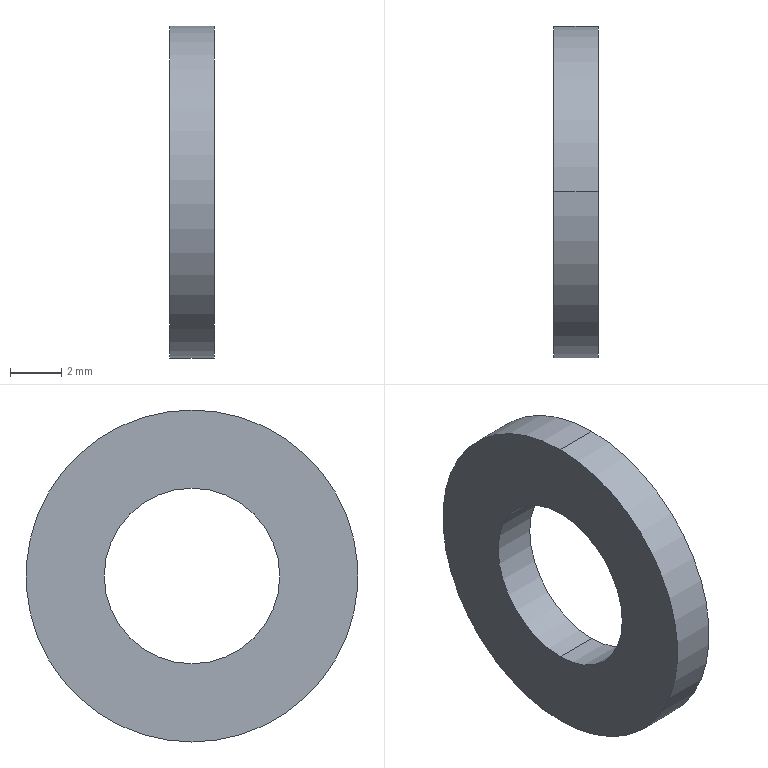Part | STEP file | flat washer narrow_am_B18.22M - Plain washer, 6 mm, narrow | 1 solid | 6 faces | box 1.75 x 13 x 13 mm | volume 167.412 mm3 | cylinder 4 | plane 2 | commonest cylinder face diameters 6.87 x2 13 x2
STEP:
#1=CARTESIAN_POINT('',(0.,0.,0.));
#2=DIRECTION('',(0.,0.,1.));
#3=DIRECTION('',(1.,0.,0.));
#4=AXIS2_PLACEMENT_3D('',#1,#2,#3);
#5=CARTESIAN_POINT('',(0.,0.,6.5));
#6=VERTEX_POINT('',#5);
#7=CARTESIAN_POINT('',(0.,0.,-6.5));
#8=VERTEX_POINT('',#7);
#9=CARTESIAN_POINT('',(0.,0.,0.));
#10=DIRECTION('',(-1.,0.,0.));
#11=DIRECTION('',(0.,0.,1.));
#12=AXIS2_PLACEMENT_3D('',#9,#10,#11);
#13=CIRCLE('',#12,6.5);
#14=CARTESIAN_POINT('',(-34.925,0.,0.));
#15=DIRECTION('',(-1.,0.,0.));
#16=DIRECTION('',(0.,0.,1.));
#17=AXIS2_PLACEMENT_3D('',#14,#15,#16);
#18=CYLINDRICAL_SURFACE('',#17,6.5);
#19=CARTESIAN_POINT('',(0.,-34.925));
#20=DIRECTION('',(1.,0.));
#21=VECTOR('',#20,1.);
#22=LINE('',#19,#21);
#23=(GEOMETRIC_REPRESENTATION_CONTEXT(2)PARAMETRIC_REPRESENTATION_CONTEXT()REPRESENTATION_CONTEXT('',''));
#24=DEFINITIONAL_REPRESENTATION('',(#22),#23);
#25=PCURVE('',#18,#24);
#26=CARTESIAN_POINT('',(0.,3.435,0.));
#27=DIRECTION('',(-1.,0.,0.));
#28=DIRECTION('',(0.,0.,1.));
#29=AXIS2_PLACEMENT_3D('',#26,#27,#28);
#30=PLANE('',#29);
#31=CARTESIAN_POINT('',(0.,-3.435));
#32=DIRECTION('',(1.,0.));
#33=AXIS2_PLACEMENT_2D('',#31,#32);
#34=CIRCLE('',#33,6.5);
#35=(GEOMETRIC_REPRESENTATION_CONTEXT(2)PARAMETRIC_REPRESENTATION_CONTEXT()REPRESENTATION_CONTEXT('',''));
#36=DEFINITIONAL_REPRESENTATION('',(#34),#35);
#37=PCURVE('',#30,#36);
#38=SURFACE_CURVE('',#13,(#25,#37),.PCURVE_S1.);
#39=EDGE_CURVE('',#6,#8,#38,.T.);
#40=ORIENTED_EDGE('',*,*,#39,.T.);
#41=CARTESIAN_POINT('',(-1.75,0.,-6.5));
#42=VERTEX_POINT('',#41);
#43=CARTESIAN_POINT('',(-34.925,0.,-6.5));
#44=DIRECTION('',(-1.,0.,0.));
#45=VECTOR('',#44,1.);
#46=LINE('',#43,#45);
#47=CARTESIAN_POINT('',(3.142,0.));
#48=DIRECTION('',(0.,1.));
#49=VECTOR('',#48,1.);
#50=LINE('',#47,#49);
#51=(GEOMETRIC_REPRESENTATION_CONTEXT(2)PARAMETRIC_REPRESENTATION_CONTEXT()REPRESENTATION_CONTEXT('',''));
#52=DEFINITIONAL_REPRESENTATION('',(#50),#51);
#53=PCURVE('',#18,#52);
#54=CARTESIAN_POINT('',(-34.925,0.,0.));
#55=DIRECTION('',(-1.,0.,0.));
#56=DIRECTION('',(0.,0.,1.));
#57=AXIS2_PLACEMENT_3D('',#54,#55,#56);
#58=CYLINDRICAL_SURFACE('',#57,6.5);
#59=CARTESIAN_POINT('',(3.142,0.));
#60=DIRECTION('',(0.,1.));
#61=VECTOR('',#60,1.);
#62=LINE('',#59,#61);
#63=(GEOMETRIC_REPRESENTATION_CONTEXT(2)PARAMETRIC_REPRESENTATION_CONTEXT()REPRESENTATION_CONTEXT('',''));
#64=DEFINITIONAL_REPRESENTATION('',(#62),#63);
#65=PCURVE('',#58,#64);
#66=SURFACE_CURVE('',#46,(#53,#65),.PCURVE_S1.);
#67=EDGE_CURVE('',#8,#42,#66,.T.);
#68=ORIENTED_EDGE('',*,*,#67,.T.);
#69=CARTESIAN_POINT('',(-1.75,0.,6.5));
#70=VERTEX_POINT('',#69);
#71=CARTESIAN_POINT('',(-1.75,0.,0.));
#72=DIRECTION('',(-1.,0.,0.));
#73=DIRECTION('',(0.,0.,1.));
#74=AXIS2_PLACEMENT_3D('',#71,#72,#73);
#75=CIRCLE('',#74,6.5);
#76=CARTESIAN_POINT('',(0.,-33.175));
#77=DIRECTION('',(1.,0.));
#78=VECTOR('',#77,1.);
#79=LINE('',#76,#78);
#80=(GEOMETRIC_REPRESENTATION_CONTEXT(2)PARAMETRIC_REPRESENTATION_CONTEXT()REPRESENTATION_CONTEXT('',''));
#81=DEFINITIONAL_REPRESENTATION('',(#79),#80);
#82=PCURVE('',#18,#81);
#83=CARTESIAN_POINT('',(-1.75,6.5,0.));
#84=DIRECTION('',(1.,0.,0.));
#85=DIRECTION('',(0.,0.,-1.));
#86=AXIS2_PLACEMENT_3D('',#83,#84,#85);
#87=PLANE('',#86);
#88=CARTESIAN_POINT('',(-6.5,-6.5));
#89=CARTESIAN_POINT('',(-6.5,4.758));
#90=CARTESIAN_POINT('',(3.25,-0.8708));
#91=CARTESIAN_POINT('',(13.,-6.5));
#92=CARTESIAN_POINT('',(3.25,-12.129));
#93=CARTESIAN_POINT('',(-6.5,-17.758));
#94=CARTESIAN_POINT('',(-6.5,-6.5));
#95=(BOUNDED_CURVE()B_SPLINE_CURVE(2,(#88,#89,#90,#91,#92,#93,#94),.UNSPECIFIED.,.T.,.F.)B_SPLINE_CURVE_WITH_KNOTS((1,2,2,2,2,1),(-2.094,0.,2.094,4.189,6.283,8.378),.UNSPECIFIED.)CURVE()GEOMETRIC_REPRESENTATION_ITEM()RATIONAL_B_SPLINE_CURVE((1.,0.5,1.,0.5,1.,0.5,1.))REPRESENTATION_ITEM(''));
#96=(GEOMETRIC_REPRESENTATION_CONTEXT(2)PARAMETRIC_REPRESENTATION_CONTEXT()REPRESENTATION_CONTEXT('',''));
#97=DEFINITIONAL_REPRESENTATION('',(#95),#96);
#98=PCURVE('',#87,#97);
#99=SURFACE_CURVE('',#75,(#82,#98),.PCURVE_S1.);
#100=EDGE_CURVE('',#70,#42,#99,.T.);
#101=ORIENTED_EDGE('',*,*,#100,.F.);
#102=CARTESIAN_POINT('',(-34.925,0.,6.5));
#103=DIRECTION('',(-1.,0.,0.));
#104=VECTOR('',#103,1.);
#105=LINE('',#102,#104);
#106=CARTESIAN_POINT('',(0.,0.));
#107=DIRECTION('',(0.,1.));
#108=VECTOR('',#107,1.);
#109=LINE('',#106,#108);
#110=(GEOMETRIC_REPRESENTATION_CONTEXT(2)PARAMETRIC_REPRESENTATION_CONTEXT()REPRESENTATION_CONTEXT('',''));
#111=DEFINITIONAL_REPRESENTATION('',(#109),#110);
#112=PCURVE('',#18,#111);
#113=CARTESIAN_POINT('',(6.283,0.));
#114=DIRECTION('',(0.,1.));
#115=VECTOR('',#114,1.);
#116=LINE('',#113,#115);
#117=(GEOMETRIC_REPRESENTATION_CONTEXT(2)PARAMETRIC_REPRESENTATION_CONTEXT()REPRESENTATION_CONTEXT('',''));
#118=DEFINITIONAL_REPRESENTATION('',(#116),#117);
#119=PCURVE('',#58,#118);
#120=SURFACE_CURVE('',#105,(#112,#119),.PCURVE_S1.);
#121=EDGE_CURVE('',#6,#70,#120,.T.);
#122=ORIENTED_EDGE('',*,*,#121,.F.);
#123=EDGE_LOOP('',(#40,#68,#101,#122));
#124=FACE_BOUND('',#123,.T.);
#125=ADVANCED_FACE('',(#124),#18,.T.);
#126=CARTESIAN_POINT('',(0.,0.,3.435));
#127=VERTEX_POINT('',#126);
#128=CARTESIAN_POINT('',(-1.75,0.,3.435));
#129=VERTEX_POINT('',#128);
#130=CARTESIAN_POINT('',(-34.925,0.,3.435));
#131=DIRECTION('',(-1.,0.,0.));
#132=VECTOR('',#131,1.);
#133=LINE('',#130,#132);
#134=CARTESIAN_POINT('',(-34.925,0.,0.));
#135=DIRECTION('',(-1.,0.,0.));
#136=DIRECTION('',(0.,0.,1.));
#137=AXIS2_PLACEMENT_3D('',#134,#135,#136);
#138=CYLINDRICAL_SURFACE('',#137,3.435);
#139=CARTESIAN_POINT('',(6.283,0.));
#140=DIRECTION('',(0.,1.));
#141=VECTOR('',#140,1.);
#142=LINE('',#139,#141);
#143=(GEOMETRIC_REPRESENTATION_CONTEXT(2)PARAMETRIC_REPRESENTATION_CONTEXT()REPRESENTATION_CONTEXT('',''));
#144=DEFINITIONAL_REPRESENTATION('',(#142),#143);
#145=PCURVE('',#138,#144);
#146=CARTESIAN_POINT('',(-34.925,0.,0.));
#147=DIRECTION('',(-1.,0.,0.));
#148=DIRECTION('',(0.,0.,1.));
#149=AXIS2_PLACEMENT_3D('',#146,#147,#148);
#150=CYLINDRICAL_SURFACE('',#149,3.435);
#151=CARTESIAN_POINT('',(0.,0.));
#152=DIRECTION('',(0.,1.));
#153=VECTOR('',#152,1.);
#154=LINE('',#151,#153);
#155=(GEOMETRIC_REPRESENTATION_CONTEXT(2)PARAMETRIC_REPRESENTATION_CONTEXT()REPRESENTATION_CONTEXT('',''));
#156=DEFINITIONAL_REPRESENTATION('',(#154),#155);
#157=PCURVE('',#150,#156);
#158=SURFACE_CURVE('',#133,(#145,#157),.PCURVE_S1.);
#159=EDGE_CURVE('',#127,#129,#158,.T.);
#160=ORIENTED_EDGE('',*,*,#159,.T.);
#161=CARTESIAN_POINT('',(-1.75,0.,-3.435));
#162=VERTEX_POINT('',#161);
#163=CARTESIAN_POINT('',(-1.75,0.,0.));
#164=DIRECTION('',(-1.,0.,0.));
#165=DIRECTION('',(0.,0.,1.));
#166=AXIS2_PLACEMENT_3D('',#163,#164,#165);
#167=CIRCLE('',#166,3.435);
#168=CARTESIAN_POINT('',(0.,-33.175));
#169=DIRECTION('',(1.,0.));
#170=VECTOR('',#169,1.);
#171=LINE('',#168,#170);
#172=(GEOMETRIC_REPRESENTATION_CONTEXT(2)PARAMETRIC_REPRESENTATION_CONTEXT()REPRESENTATION_CONTEXT('',''));
#173=DEFINITIONAL_REPRESENTATION('',(#171),#172);
#174=PCURVE('',#138,#173);
#175=CARTESIAN_POINT('',(-3.435,-6.5));
#176=CARTESIAN_POINT('',(-3.435,-0.5504));
#177=CARTESIAN_POINT('',(1.718,-3.525));
#178=CARTESIAN_POINT('',(6.87,-6.5));
#179=CARTESIAN_POINT('',(1.718,-9.475));
#180=CARTESIAN_POINT('',(-3.435,-12.45));
#181=CARTESIAN_POINT('',(-3.435,-6.5));
#182=(BOUNDED_CURVE()B_SPLINE_CURVE(2,(#175,#176,#177,#178,#179,#180,#181),.UNSPECIFIED.,.T.,.F.)B_SPLINE_CURVE_WITH_KNOTS((1,2,2,2,2,1),(-2.094,0.,2.094,4.189,6.283,8.378),.UNSPECIFIED.)CURVE()GEOMETRIC_REPRESENTATION_ITEM()RATIONAL_B_SPLINE_CURVE((1.,0.5,1.,0.5,1.,0.5,1.))REPRESENTATION_ITEM(''));
#183=(GEOMETRIC_REPRESENTATION_CONTEXT(2)PARAMETRIC_REPRESENTATION_CONTEXT()REPRESENTATION_CONTEXT('',''));
#184=DEFINITIONAL_REPRESENTATION('',(#182),#183);
#185=PCURVE('',#87,#184);
#186=SURFACE_CURVE('',#167,(#174,#185),.PCURVE_S1.);
#187=EDGE_CURVE('',#162,#129,#186,.T.);
#188=ORIENTED_EDGE('',*,*,#187,.F.);
#189=CARTESIAN_POINT('',(0.,0.,-3.435));
#190=VERTEX_POINT('',#189);
#191=CARTESIAN_POINT('',(-34.925,0.,-3.435));
#192=DIRECTION('',(-1.,0.,0.));
#193=VECTOR('',#192,1.);
#194=LINE('',#191,#193);
#195=CARTESIAN_POINT('',(3.142,0.));
#196=DIRECTION('',(0.,1.));
#197=VECTOR('',#196,1.);
#198=LINE('',#195,#197);
#199=(GEOMETRIC_REPRESENTATION_CONTEXT(2)PARAMETRIC_REPRESENTATION_CONTEXT()REPRESENTATION_CONTEXT('',''));
#200=DEFINITIONAL_REPRESENTATION('',(#198),#199);
#201=PCURVE('',#138,#200);
#202=CARTESIAN_POINT('',(3.142,0.));
#203=DIRECTION('',(0.,1.));
#204=VECTOR('',#203,1.);
#205=LINE('',#202,#204);
#206=(GEOMETRIC_REPRESENTATION_CONTEXT(2)PARAMETRIC_REPRESENTATION_CONTEXT()REPRESENTATION_CONTEXT('',''));
#207=DEFINITIONAL_REPRESENTATION('',(#205),#206);
#208=PCURVE('',#150,#207);
#209=SURFACE_CURVE('',#194,(#201,#208),.PCURVE_S1.);
#210=EDGE_CURVE('',#190,#162,#209,.T.);
#211=ORIENTED_EDGE('',*,*,#210,.F.);
#212=CARTESIAN_POINT('',(0.,0.,0.));
#213=DIRECTION('',(-1.,0.,0.));
#214=DIRECTION('',(0.,0.,1.));
#215=AXIS2_PLACEMENT_3D('',#212,#213,#214);
#216=CIRCLE('',#215,3.435);
#217=CARTESIAN_POINT('',(0.,-34.925));
#218=DIRECTION('',(1.,0.));
#219=VECTOR('',#218,1.);
#220=LINE('',#217,#219);
#221=(GEOMETRIC_REPRESENTATION_CONTEXT(2)PARAMETRIC_REPRESENTATION_CONTEXT()REPRESENTATION_CONTEXT('',''));
#222=DEFINITIONAL_REPRESENTATION('',(#220),#221);
#223=PCURVE('',#138,#222);
#224=CARTESIAN_POINT('',(0.,-3.435));
#225=DIRECTION('',(1.,0.));
#226=AXIS2_PLACEMENT_2D('',#224,#225);
#227=CIRCLE('',#226,3.435);
#228=(GEOMETRIC_REPRESENTATION_CONTEXT(2)PARAMETRIC_REPRESENTATION_CONTEXT()REPRESENTATION_CONTEXT('',''));
#229=DEFINITIONAL_REPRESENTATION('',(#227),#228);
#230=PCURVE('',#30,#229);
#231=SURFACE_CURVE('',#216,(#223,#230),.PCURVE_S1.);
#232=EDGE_CURVE('',#190,#127,#231,.T.);
#233=ORIENTED_EDGE('',*,*,#232,.T.);
#234=EDGE_LOOP('',(#160,#188,#211,#233));
#235=FACE_BOUND('',#234,.F.);
#236=ADVANCED_FACE('',(#235),#138,.F.);
#237=CARTESIAN_POINT('',(-1.75,0.,0.));
#238=DIRECTION('',(-1.,0.,0.));
#239=DIRECTION('',(0.,0.,1.));
#240=AXIS2_PLACEMENT_3D('',#237,#238,#239);
#241=CIRCLE('',#240,3.435);
#242=CARTESIAN_POINT('',(0.,-33.175));
#243=DIRECTION('',(1.,0.));
#244=VECTOR('',#243,1.);
#245=LINE('',#242,#244);
#246=(GEOMETRIC_REPRESENTATION_CONTEXT(2)PARAMETRIC_REPRESENTATION_CONTEXT()REPRESENTATION_CONTEXT('',''));
#247=DEFINITIONAL_REPRESENTATION('',(#245),#246);
#248=PCURVE('',#150,#247);
#249=CARTESIAN_POINT('',(-3.435,-6.5));
#250=CARTESIAN_POINT('',(-3.435,-0.5504));
#251=CARTESIAN_POINT('',(1.718,-3.525));
#252=CARTESIAN_POINT('',(6.87,-6.5));
#253=CARTESIAN_POINT('',(1.718,-9.475));
#254=CARTESIAN_POINT('',(-3.435,-12.45));
#255=CARTESIAN_POINT('',(-3.435,-6.5));
#256=(BOUNDED_CURVE()B_SPLINE_CURVE(2,(#249,#250,#251,#252,#253,#254,#255),.UNSPECIFIED.,.T.,.F.)B_SPLINE_CURVE_WITH_KNOTS((1,2,2,2,2,1),(-2.094,0.,2.094,4.189,6.283,8.378),.UNSPECIFIED.)CURVE()GEOMETRIC_REPRESENTATION_ITEM()RATIONAL_B_SPLINE_CURVE((1.,0.5,1.,0.5,1.,0.5,1.))REPRESENTATION_ITEM(''));
#257=(GEOMETRIC_REPRESENTATION_CONTEXT(2)PARAMETRIC_REPRESENTATION_CONTEXT()REPRESENTATION_CONTEXT('',''));
#258=DEFINITIONAL_REPRESENTATION('',(#256),#257);
#259=PCURVE('',#87,#258);
#260=SURFACE_CURVE('',#241,(#248,#259),.PCURVE_S1.);
#261=EDGE_CURVE('',#129,#162,#260,.T.);
#262=ORIENTED_EDGE('',*,*,#261,.F.);
#263=ORIENTED_EDGE('',*,*,#159,.F.);
#264=CARTESIAN_POINT('',(0.,0.,0.));
#265=DIRECTION('',(-1.,0.,0.));
#266=DIRECTION('',(0.,0.,1.));
#267=AXIS2_PLACEMENT_3D('',#264,#265,#266);
#268=CIRCLE('',#267,3.435);
#269=CARTESIAN_POINT('',(0.,-34.925));
#270=DIRECTION('',(1.,0.));
#271=VECTOR('',#270,1.);
#272=LINE('',#269,#271);
#273=(GEOMETRIC_REPRESENTATION_CONTEXT(2)PARAMETRIC_REPRESENTATION_CONTEXT()REPRESENTATION_CONTEXT('',''));
#274=DEFINITIONAL_REPRESENTATION('',(#272),#273);
#275=PCURVE('',#150,#274);
#276=CARTESIAN_POINT('',(0.,-3.435));
#277=DIRECTION('',(1.,0.));
#278=AXIS2_PLACEMENT_2D('',#276,#277);
#279=CIRCLE('',#278,3.435);
#280=(GEOMETRIC_REPRESENTATION_CONTEXT(2)PARAMETRIC_REPRESENTATION_CONTEXT()REPRESENTATION_CONTEXT('',''));
#281=DEFINITIONAL_REPRESENTATION('',(#279),#280);
#282=PCURVE('',#30,#281);
#283=SURFACE_CURVE('',#268,(#275,#282),.PCURVE_S1.);
#284=EDGE_CURVE('',#127,#190,#283,.T.);
#285=ORIENTED_EDGE('',*,*,#284,.T.);
#286=ORIENTED_EDGE('',*,*,#210,.T.);
#287=EDGE_LOOP('',(#262,#263,#285,#286));
#288=FACE_BOUND('',#287,.F.);
#289=ADVANCED_FACE('',(#288),#150,.F.);
#290=ORIENTED_EDGE('',*,*,#39,.F.);
#291=CARTESIAN_POINT('',(0.,0.,0.));
#292=DIRECTION('',(-1.,0.,0.));
#293=DIRECTION('',(0.,0.,1.));
#294=AXIS2_PLACEMENT_3D('',#291,#292,#293);
#295=CIRCLE('',#294,6.5);
#296=CARTESIAN_POINT('',(0.,-3.435));
#297=DIRECTION('',(1.,0.));
#298=AXIS2_PLACEMENT_2D('',#296,#297);
#299=CIRCLE('',#298,6.5);
#300=(GEOMETRIC_REPRESENTATION_CONTEXT(2)PARAMETRIC_REPRESENTATION_CONTEXT()REPRESENTATION_CONTEXT('',''));
#301=DEFINITIONAL_REPRESENTATION('',(#299),#300);
#302=PCURVE('',#30,#301);
#303=CARTESIAN_POINT('',(0.,-34.925));
#304=DIRECTION('',(1.,0.));
#305=VECTOR('',#304,1.);
#306=LINE('',#303,#305);
#307=(GEOMETRIC_REPRESENTATION_CONTEXT(2)PARAMETRIC_REPRESENTATION_CONTEXT()REPRESENTATION_CONTEXT('',''));
#308=DEFINITIONAL_REPRESENTATION('',(#306),#307);
#309=PCURVE('',#58,#308);
#310=SURFACE_CURVE('',#295,(#302,#309),.PCURVE_S1.);
#311=EDGE_CURVE('',#8,#6,#310,.T.);
#312=ORIENTED_EDGE('',*,*,#311,.F.);
#313=EDGE_LOOP('',(#290,#312));
#314=FACE_BOUND('',#313,.T.);
#315=ORIENTED_EDGE('',*,*,#284,.T.);
#316=ORIENTED_EDGE('',*,*,#232,.T.);
#317=EDGE_LOOP('',(#315,#316));
#318=FACE_BOUND('',#317,.T.);
#319=ADVANCED_FACE('',(#314,#318),#30,.F.);
#320=ORIENTED_EDGE('',*,*,#67,.F.);
#321=ORIENTED_EDGE('',*,*,#311,.T.);
#322=ORIENTED_EDGE('',*,*,#121,.T.);
#323=CARTESIAN_POINT('',(-1.75,0.,0.));
#324=DIRECTION('',(-1.,0.,0.));
#325=DIRECTION('',(0.,0.,1.));
#326=AXIS2_PLACEMENT_3D('',#323,#324,#325);
#327=CIRCLE('',#326,6.5);
#328=CARTESIAN_POINT('',(0.,-33.175));
#329=DIRECTION('',(1.,0.));
#330=VECTOR('',#329,1.);
#331=LINE('',#328,#330);
#332=(GEOMETRIC_REPRESENTATION_CONTEXT(2)PARAMETRIC_REPRESENTATION_CONTEXT()REPRESENTATION_CONTEXT('',''));
#333=DEFINITIONAL_REPRESENTATION('',(#331),#332);
#334=PCURVE('',#58,#333);
#335=CARTESIAN_POINT('',(-6.5,-6.5));
#336=CARTESIAN_POINT('',(-6.5,4.758));
#337=CARTESIAN_POINT('',(3.25,-0.8708));
#338=CARTESIAN_POINT('',(13.,-6.5));
#339=CARTESIAN_POINT('',(3.25,-12.129));
#340=CARTESIAN_POINT('',(-6.5,-17.758));
#341=CARTESIAN_POINT('',(-6.5,-6.5));
#342=(BOUNDED_CURVE()B_SPLINE_CURVE(2,(#335,#336,#337,#338,#339,#340,#341),.UNSPECIFIED.,.T.,.F.)B_SPLINE_CURVE_WITH_KNOTS((1,2,2,2,2,1),(-2.094,0.,2.094,4.189,6.283,8.378),.UNSPECIFIED.)CURVE()GEOMETRIC_REPRESENTATION_ITEM()RATIONAL_B_SPLINE_CURVE((1.,0.5,1.,0.5,1.,0.5,1.))REPRESENTATION_ITEM(''));
#343=(GEOMETRIC_REPRESENTATION_CONTEXT(2)PARAMETRIC_REPRESENTATION_CONTEXT()REPRESENTATION_CONTEXT('',''));
#344=DEFINITIONAL_REPRESENTATION('',(#342),#343);
#345=PCURVE('',#87,#344);
#346=SURFACE_CURVE('',#327,(#334,#345),.PCURVE_S1.);
#347=EDGE_CURVE('',#42,#70,#346,.T.);
#348=ORIENTED_EDGE('',*,*,#347,.F.);
#349=EDGE_LOOP('',(#320,#321,#322,#348));
#350=FACE_BOUND('',#349,.T.);
#351=ADVANCED_FACE('',(#350),#58,.T.);
#352=ORIENTED_EDGE('',*,*,#261,.F.);
#353=ORIENTED_EDGE('',*,*,#187,.F.);
#354=EDGE_LOOP('',(#352,#353));
#355=FACE_BOUND('',#354,.T.);
#356=ORIENTED_EDGE('',*,*,#100,.T.);
#357=ORIENTED_EDGE('',*,*,#347,.T.);
#358=EDGE_LOOP('',(#356,#357));
#359=FACE_BOUND('',#358,.T.);
#360=ADVANCED_FACE('',(#355,#359),#87,.F.);
#361=CLOSED_SHELL('',(#125,#236,#289,#319,#351,#360));
#362=MANIFOLD_SOLID_BREP('',#361);
#363=(LENGTH_UNIT()NAMED_UNIT(*)SI_UNIT(.MILLI.,.METRE.));
#364=UNCERTAINTY_MEASURE_WITH_UNIT(LENGTH_MEASURE(0.0000001),#363,'','');
#365=(NAMED_UNIT(*)PLANE_ANGLE_UNIT()SI_UNIT($,.RADIAN.));
#366=(NAMED_UNIT(*)SI_UNIT($,.STERADIAN.)SOLID_ANGLE_UNIT());
#367=(GEOMETRIC_REPRESENTATION_CONTEXT(3)GLOBAL_UNCERTAINTY_ASSIGNED_CONTEXT((#364))GLOBAL_UNIT_ASSIGNED_CONTEXT((#363,#365,#366))REPRESENTATION_CONTEXT('',''));
#368=ADVANCED_BREP_SHAPE_REPRESENTATION('',(#4,#362),#367);